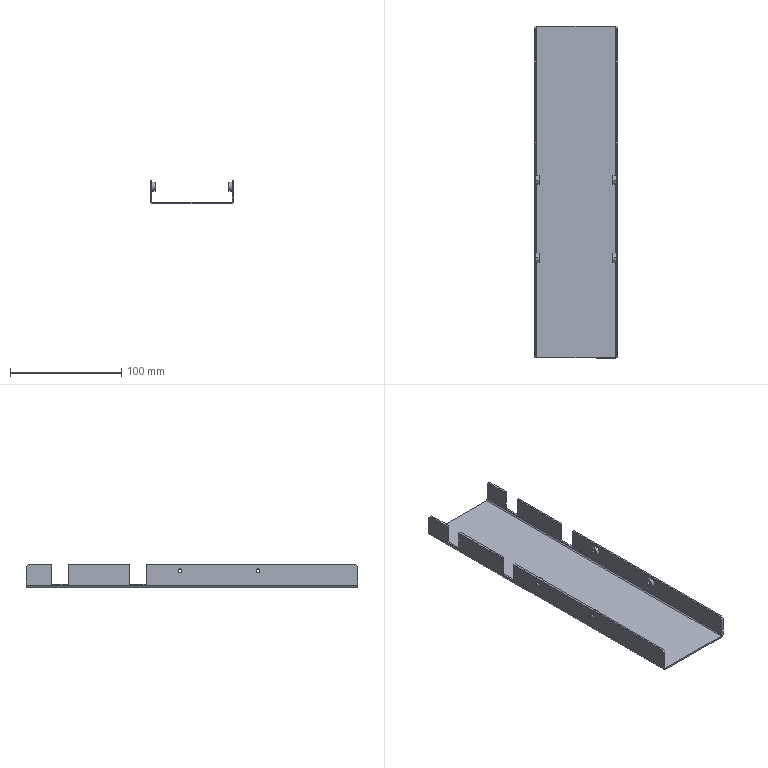Part | SolidWorks | features Chamfer 1, Cut 1, EdgeFlange 1, FlatPattern 1, HoleWzd 1, ICE 1, MirrorPattern 1, SMBaseFlange 1, SheetMetal 1 | 1 solid | 62 faces | box 75.5 x 298.5 x 21.5 mm | volume 49860 mm3 | plane 42 | cylinder 20 | commonest cylinder face diameters 3.3 x8 8 x8 2 x2 5 x2